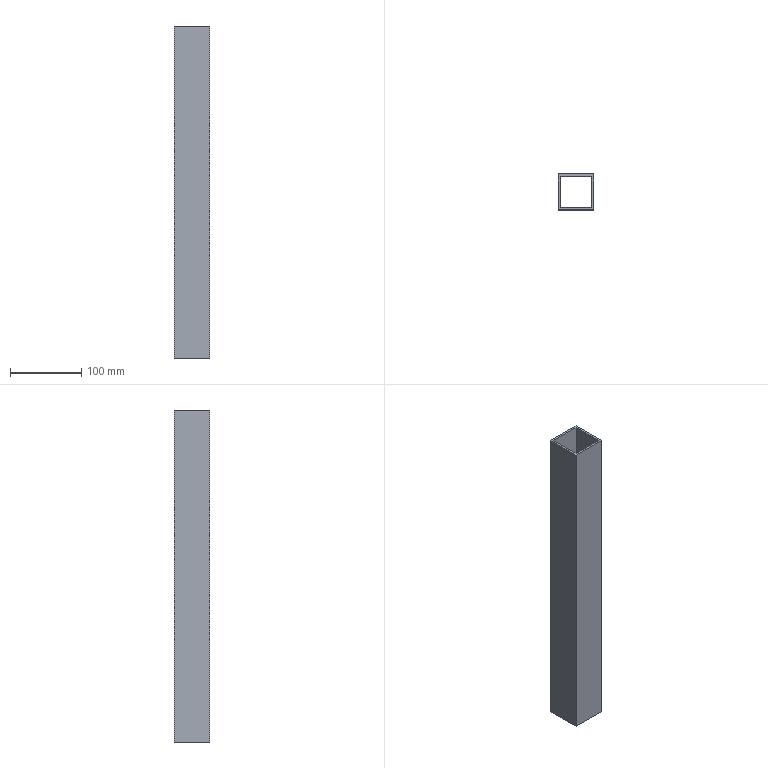Part | SolidWorks | features Extrusion 1 | 1 solid | 10 faces | box 50 x 50 x 465 mm | volume 262260 mm3 | plane 10
STEP:
#1=CARTESIAN_POINT('',(0.,0.,465.));
#2=VERTEX_POINT('',#1);
#3=CARTESIAN_POINT('',(50.,0.,465.));
#4=VERTEX_POINT('',#3);
#5=CARTESIAN_POINT('',(50.,0.,465.));
#6=DIRECTION('',(1.,0.,0.));
#7=VECTOR('',#6,1000.);
#8=LINE('',#5,#7);
#9=EDGE_CURVE('',#2,#4,#8,.T.);
#10=ORIENTED_EDGE('',*,*,#9,.T.);
#11=CARTESIAN_POINT('',(50.,50.,465.));
#12=VERTEX_POINT('',#11);
#13=CARTESIAN_POINT('',(50.,50.,465.));
#14=DIRECTION('',(0.,1.,0.));
#15=VECTOR('',#14,1000.);
#16=LINE('',#13,#15);
#17=EDGE_CURVE('',#4,#12,#16,.T.);
#18=ORIENTED_EDGE('',*,*,#17,.T.);
#19=CARTESIAN_POINT('',(0.,50.,465.));
#20=VERTEX_POINT('',#19);
#21=CARTESIAN_POINT('',(0.,50.,465.));
#22=DIRECTION('',(-1.,0.,0.));
#23=VECTOR('',#22,1000.);
#24=LINE('',#21,#23);
#25=EDGE_CURVE('',#12,#20,#24,.T.);
#26=ORIENTED_EDGE('',*,*,#25,.T.);
#27=CARTESIAN_POINT('',(0.,0.,465.));
#28=DIRECTION('',(0.,-1.,0.));
#29=VECTOR('',#28,1000.);
#30=LINE('',#27,#29);
#31=EDGE_CURVE('',#20,#2,#30,.T.);
#32=ORIENTED_EDGE('',*,*,#31,.T.);
#33=EDGE_LOOP('',(#10,#18,#26,#32));
#34=FACE_OUTER_BOUND('',#33,.T.);
#35=CARTESIAN_POINT('',(3.,3.,465.));
#36=VERTEX_POINT('',#35);
#37=CARTESIAN_POINT('',(47.,3.,465.));
#38=VERTEX_POINT('',#37);
#39=CARTESIAN_POINT('',(47.,3.,465.));
#40=DIRECTION('',(1.,0.,0.));
#41=VECTOR('',#40,1000.);
#42=LINE('',#39,#41);
#43=EDGE_CURVE('',#36,#38,#42,.T.);
#44=ORIENTED_EDGE('',*,*,#43,.F.);
#45=CARTESIAN_POINT('',(3.,47.,465.));
#46=VERTEX_POINT('',#45);
#47=CARTESIAN_POINT('',(3.,3.,465.));
#48=DIRECTION('',(0.,-1.,0.));
#49=VECTOR('',#48,1000.);
#50=LINE('',#47,#49);
#51=EDGE_CURVE('',#46,#36,#50,.T.);
#52=ORIENTED_EDGE('',*,*,#51,.F.);
#53=CARTESIAN_POINT('',(47.,47.,465.));
#54=VERTEX_POINT('',#53);
#55=CARTESIAN_POINT('',(3.,47.,465.));
#56=DIRECTION('',(-1.,0.,0.));
#57=VECTOR('',#56,1000.);
#58=LINE('',#55,#57);
#59=EDGE_CURVE('',#54,#46,#58,.T.);
#60=ORIENTED_EDGE('',*,*,#59,.F.);
#61=CARTESIAN_POINT('',(47.,47.,465.));
#62=DIRECTION('',(0.,1.,0.));
#63=VECTOR('',#62,1000.);
#64=LINE('',#61,#63);
#65=EDGE_CURVE('',#38,#54,#64,.T.);
#66=ORIENTED_EDGE('',*,*,#65,.F.);
#67=EDGE_LOOP('',(#44,#52,#60,#66));
#68=FACE_BOUND('',#67,.T.);
#69=CARTESIAN_POINT('',(0.,0.,465.));
#70=DIRECTION('',(0.,0.,-1.));
#71=DIRECTION('',(-1.,0.,0.));
#72=AXIS2_PLACEMENT_3D('',#69,#70,#71);
#73=PLANE('',#72);
#74=ADVANCED_FACE('',(#34,#68),#73,.F.);
#75=CARTESIAN_POINT('',(0.,0.,0.));
#76=VERTEX_POINT('',#75);
#77=CARTESIAN_POINT('',(50.,0.,0.));
#78=VERTEX_POINT('',#77);
#79=CARTESIAN_POINT('',(50.,0.,0.));
#80=DIRECTION('',(1.,0.,0.));
#81=VECTOR('',#80,1000.);
#82=LINE('',#79,#81);
#83=EDGE_CURVE('',#76,#78,#82,.T.);
#84=ORIENTED_EDGE('',*,*,#83,.F.);
#85=CARTESIAN_POINT('',(0.,50.,0.));
#86=VERTEX_POINT('',#85);
#87=CARTESIAN_POINT('',(0.,0.,0.));
#88=DIRECTION('',(0.,-1.,0.));
#89=VECTOR('',#88,1000.);
#90=LINE('',#87,#89);
#91=EDGE_CURVE('',#86,#76,#90,.T.);
#92=ORIENTED_EDGE('',*,*,#91,.F.);
#93=CARTESIAN_POINT('',(50.,50.,0.));
#94=VERTEX_POINT('',#93);
#95=CARTESIAN_POINT('',(0.,50.,0.));
#96=DIRECTION('',(-1.,0.,0.));
#97=VECTOR('',#96,1000.);
#98=LINE('',#95,#97);
#99=EDGE_CURVE('',#94,#86,#98,.T.);
#100=ORIENTED_EDGE('',*,*,#99,.F.);
#101=CARTESIAN_POINT('',(50.,50.,0.));
#102=DIRECTION('',(0.,1.,0.));
#103=VECTOR('',#102,1000.);
#104=LINE('',#101,#103);
#105=EDGE_CURVE('',#78,#94,#104,.T.);
#106=ORIENTED_EDGE('',*,*,#105,.F.);
#107=EDGE_LOOP('',(#84,#92,#100,#106));
#108=FACE_OUTER_BOUND('',#107,.T.);
#109=CARTESIAN_POINT('',(3.,47.,0.));
#110=VERTEX_POINT('',#109);
#111=CARTESIAN_POINT('',(3.,3.,0.));
#112=VERTEX_POINT('',#111);
#113=CARTESIAN_POINT('',(3.,3.,0.));
#114=DIRECTION('',(0.,-1.,0.));
#115=VECTOR('',#114,1000.);
#116=LINE('',#113,#115);
#117=EDGE_CURVE('',#110,#112,#116,.T.);
#118=ORIENTED_EDGE('',*,*,#117,.T.);
#119=CARTESIAN_POINT('',(47.,3.,0.));
#120=VERTEX_POINT('',#119);
#121=CARTESIAN_POINT('',(47.,3.,0.));
#122=DIRECTION('',(1.,0.,0.));
#123=VECTOR('',#122,1000.);
#124=LINE('',#121,#123);
#125=EDGE_CURVE('',#112,#120,#124,.T.);
#126=ORIENTED_EDGE('',*,*,#125,.T.);
#127=CARTESIAN_POINT('',(47.,47.,0.));
#128=VERTEX_POINT('',#127);
#129=CARTESIAN_POINT('',(47.,47.,0.));
#130=DIRECTION('',(0.,1.,0.));
#131=VECTOR('',#130,1000.);
#132=LINE('',#129,#131);
#133=EDGE_CURVE('',#120,#128,#132,.T.);
#134=ORIENTED_EDGE('',*,*,#133,.T.);
#135=CARTESIAN_POINT('',(3.,47.,0.));
#136=DIRECTION('',(-1.,0.,0.));
#137=VECTOR('',#136,1000.);
#138=LINE('',#135,#137);
#139=EDGE_CURVE('',#128,#110,#138,.T.);
#140=ORIENTED_EDGE('',*,*,#139,.T.);
#141=EDGE_LOOP('',(#118,#126,#134,#140));
#142=FACE_BOUND('',#141,.T.);
#143=CARTESIAN_POINT('',(0.,0.,0.));
#144=DIRECTION('',(0.,0.,-1.));
#145=DIRECTION('',(-1.,0.,0.));
#146=AXIS2_PLACEMENT_3D('',#143,#144,#145);
#147=PLANE('',#146);
#148=ADVANCED_FACE('',(#108,#142),#147,.T.);
#149=ORIENTED_EDGE('',*,*,#83,.T.);
#150=CARTESIAN_POINT('',(50.,0.,465.));
#151=DIRECTION('',(0.,0.,-1.));
#152=VECTOR('',#151,1000.);
#153=LINE('',#150,#152);
#154=EDGE_CURVE('',#4,#78,#153,.T.);
#155=ORIENTED_EDGE('',*,*,#154,.F.);
#156=ORIENTED_EDGE('',*,*,#9,.F.);
#157=CARTESIAN_POINT('',(0.,0.,465.));
#158=DIRECTION('',(0.,0.,-1.));
#159=VECTOR('',#158,1000.);
#160=LINE('',#157,#159);
#161=EDGE_CURVE('',#2,#76,#160,.T.);
#162=ORIENTED_EDGE('',*,*,#161,.T.);
#163=EDGE_LOOP('',(#149,#155,#156,#162));
#164=FACE_OUTER_BOUND('',#163,.T.);
#165=CARTESIAN_POINT('',(50.,0.,465.));
#166=DIRECTION('',(0.,1.,0.));
#167=DIRECTION('',(0.,0.,1.));
#168=AXIS2_PLACEMENT_3D('',#165,#166,#167);
#169=PLANE('',#168);
#170=ADVANCED_FACE('',(#164),#169,.F.);
#171=ORIENTED_EDGE('',*,*,#105,.T.);
#172=CARTESIAN_POINT('',(50.,50.,465.));
#173=DIRECTION('',(0.,0.,-1.));
#174=VECTOR('',#173,1000.);
#175=LINE('',#172,#174);
#176=EDGE_CURVE('',#12,#94,#175,.T.);
#177=ORIENTED_EDGE('',*,*,#176,.F.);
#178=ORIENTED_EDGE('',*,*,#17,.F.);
#179=ORIENTED_EDGE('',*,*,#154,.T.);
#180=EDGE_LOOP('',(#171,#177,#178,#179));
#181=FACE_OUTER_BOUND('',#180,.T.);
#182=CARTESIAN_POINT('',(50.,50.,465.));
#183=DIRECTION('',(-1.,0.,0.));
#184=DIRECTION('',(0.,0.,1.));
#185=AXIS2_PLACEMENT_3D('',#182,#183,#184);
#186=PLANE('',#185);
#187=ADVANCED_FACE('',(#181),#186,.F.);
#188=ORIENTED_EDGE('',*,*,#99,.T.);
#189=CARTESIAN_POINT('',(0.,50.,465.));
#190=DIRECTION('',(0.,0.,-1.));
#191=VECTOR('',#190,1000.);
#192=LINE('',#189,#191);
#193=EDGE_CURVE('',#20,#86,#192,.T.);
#194=ORIENTED_EDGE('',*,*,#193,.F.);
#195=ORIENTED_EDGE('',*,*,#25,.F.);
#196=ORIENTED_EDGE('',*,*,#176,.T.);
#197=EDGE_LOOP('',(#188,#194,#195,#196));
#198=FACE_OUTER_BOUND('',#197,.T.);
#199=CARTESIAN_POINT('',(0.,50.,465.));
#200=DIRECTION('',(0.,-1.,0.));
#201=DIRECTION('',(0.,0.,-1.));
#202=AXIS2_PLACEMENT_3D('',#199,#200,#201);
#203=PLANE('',#202);
#204=ADVANCED_FACE('',(#198),#203,.F.);
#205=ORIENTED_EDGE('',*,*,#91,.T.);
#206=ORIENTED_EDGE('',*,*,#161,.F.);
#207=ORIENTED_EDGE('',*,*,#31,.F.);
#208=ORIENTED_EDGE('',*,*,#193,.T.);
#209=EDGE_LOOP('',(#205,#206,#207,#208));
#210=FACE_OUTER_BOUND('',#209,.T.);
#211=CARTESIAN_POINT('',(0.,0.,465.));
#212=DIRECTION('',(1.,0.,0.));
#213=DIRECTION('',(0.,0.,-1.));
#214=AXIS2_PLACEMENT_3D('',#211,#212,#213);
#215=PLANE('',#214);
#216=ADVANCED_FACE('',(#210),#215,.F.);
#217=ORIENTED_EDGE('',*,*,#125,.F.);
#218=CARTESIAN_POINT('',(3.,3.,465.));
#219=DIRECTION('',(0.,0.,-1.));
#220=VECTOR('',#219,1000.);
#221=LINE('',#218,#220);
#222=EDGE_CURVE('',#36,#112,#221,.T.);
#223=ORIENTED_EDGE('',*,*,#222,.F.);
#224=ORIENTED_EDGE('',*,*,#43,.T.);
#225=CARTESIAN_POINT('',(47.,3.,465.));
#226=DIRECTION('',(0.,0.,-1.));
#227=VECTOR('',#226,1000.);
#228=LINE('',#225,#227);
#229=EDGE_CURVE('',#38,#120,#228,.T.);
#230=ORIENTED_EDGE('',*,*,#229,.T.);
#231=EDGE_LOOP('',(#217,#223,#224,#230));
#232=FACE_OUTER_BOUND('',#231,.T.);
#233=CARTESIAN_POINT('',(47.,3.,465.));
#234=DIRECTION('',(0.,1.,0.));
#235=DIRECTION('',(0.,0.,1.));
#236=AXIS2_PLACEMENT_3D('',#233,#234,#235);
#237=PLANE('',#236);
#238=ADVANCED_FACE('',(#232),#237,.T.);
#239=ORIENTED_EDGE('',*,*,#133,.F.);
#240=ORIENTED_EDGE('',*,*,#229,.F.);
#241=ORIENTED_EDGE('',*,*,#65,.T.);
#242=CARTESIAN_POINT('',(47.,47.,465.));
#243=DIRECTION('',(0.,0.,-1.));
#244=VECTOR('',#243,1000.);
#245=LINE('',#242,#244);
#246=EDGE_CURVE('',#54,#128,#245,.T.);
#247=ORIENTED_EDGE('',*,*,#246,.T.);
#248=EDGE_LOOP('',(#239,#240,#241,#247));
#249=FACE_OUTER_BOUND('',#248,.T.);
#250=CARTESIAN_POINT('',(47.,47.,465.));
#251=DIRECTION('',(-1.,0.,0.));
#252=DIRECTION('',(0.,0.,1.));
#253=AXIS2_PLACEMENT_3D('',#250,#251,#252);
#254=PLANE('',#253);
#255=ADVANCED_FACE('',(#249),#254,.T.);
#256=ORIENTED_EDGE('',*,*,#139,.F.);
#257=ORIENTED_EDGE('',*,*,#246,.F.);
#258=ORIENTED_EDGE('',*,*,#59,.T.);
#259=CARTESIAN_POINT('',(3.,47.,465.));
#260=DIRECTION('',(0.,0.,-1.));
#261=VECTOR('',#260,1000.);
#262=LINE('',#259,#261);
#263=EDGE_CURVE('',#46,#110,#262,.T.);
#264=ORIENTED_EDGE('',*,*,#263,.T.);
#265=EDGE_LOOP('',(#256,#257,#258,#264));
#266=FACE_OUTER_BOUND('',#265,.T.);
#267=CARTESIAN_POINT('',(3.,47.,465.));
#268=DIRECTION('',(0.,-1.,0.));
#269=DIRECTION('',(0.,0.,-1.));
#270=AXIS2_PLACEMENT_3D('',#267,#268,#269);
#271=PLANE('',#270);
#272=ADVANCED_FACE('',(#266),#271,.T.);
#273=ORIENTED_EDGE('',*,*,#117,.F.);
#274=ORIENTED_EDGE('',*,*,#263,.F.);
#275=ORIENTED_EDGE('',*,*,#51,.T.);
#276=ORIENTED_EDGE('',*,*,#222,.T.);
#277=EDGE_LOOP('',(#273,#274,#275,#276));
#278=FACE_OUTER_BOUND('',#277,.T.);
#279=CARTESIAN_POINT('',(3.,3.,465.));
#280=DIRECTION('',(1.,0.,0.));
#281=DIRECTION('',(0.,0.,-1.));
#282=AXIS2_PLACEMENT_3D('',#279,#280,#281);
#283=PLANE('',#282);
#284=ADVANCED_FACE('',(#278),#283,.T.);
#285=CLOSED_SHELL('',(#74,#148,#170,#187,#204,#216,#238,#255,#272,#284));
#286=MANIFOLD_SOLID_BREP('',#285);
#287=CARTESIAN_POINT('',(0.,0.,0.));
#288=DIRECTION('',(0.,0.,1.));
#289=DIRECTION('',(1.,0.,0.));
#290=AXIS2_PLACEMENT_3D('',#287,#288,#289);
#291=(LENGTH_UNIT()NAMED_UNIT(*)SI_UNIT(.MILLI.,.METRE.));
#292=UNCERTAINTY_MEASURE_WITH_UNIT(LENGTH_MEASURE(0.00001),#291,'','');
#293=(NAMED_UNIT(*)PLANE_ANGLE_UNIT()SI_UNIT($,.RADIAN.));
#294=(NAMED_UNIT(*)SI_UNIT($,.STERADIAN.)SOLID_ANGLE_UNIT());
#295=(GEOMETRIC_REPRESENTATION_CONTEXT(3)GLOBAL_UNCERTAINTY_ASSIGNED_CONTEXT((#292))GLOBAL_UNIT_ASSIGNED_CONTEXT((#291,#293,#294))REPRESENTATION_CONTEXT('',''));
#296=ADVANCED_BREP_SHAPE_REPRESENTATION('',(#286,#290),#295);